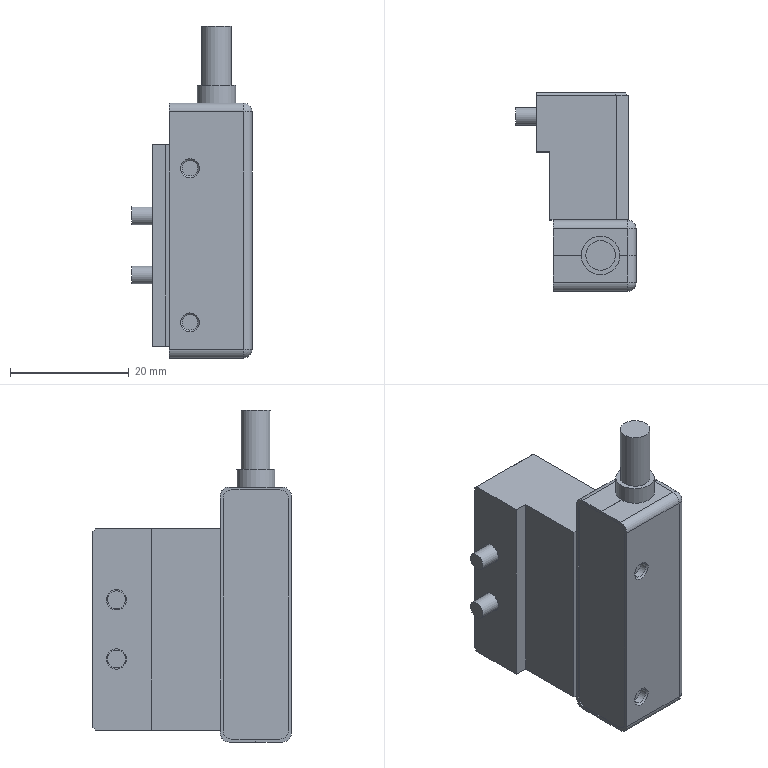Part | STEP file | BODY7_E-RAM6-S-640-ME30-C5 | 1 solid | 146 faces | box 20.3 x 33.5 x 56 mm | volume 16364 mm3 | plane 96 | cylinder 35 | cone 7 | torus 4 | sphere 4 | commonest cylinder face diameters 3 x16 5.5 x4 6 x4 2.6 x2 2.998 x2 3.4 x2